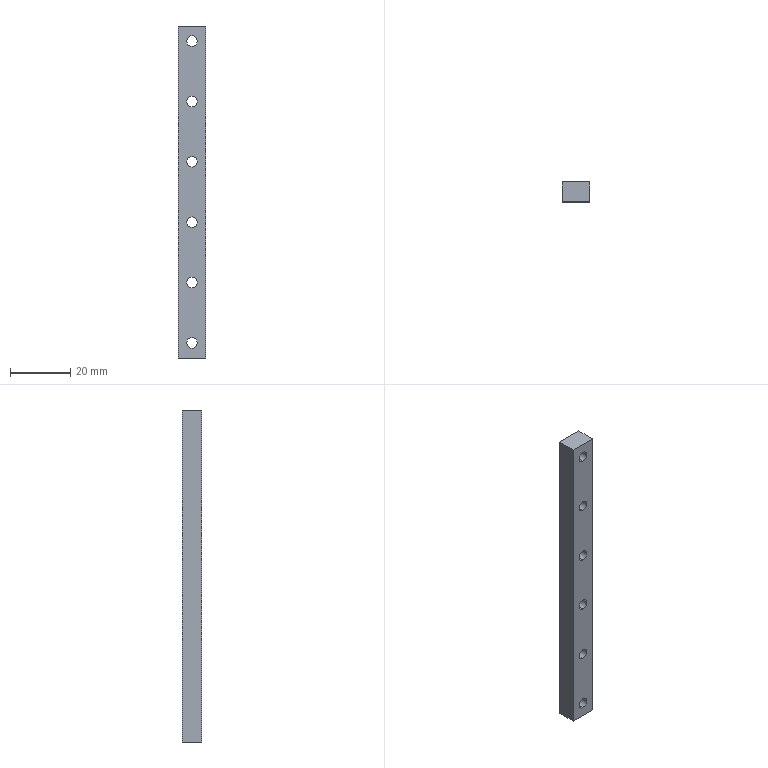Part | STEP file | Mount electronic clip sMGN9C110 | 1 solid | 36 faces | box 9 x 6.5 x 110 mm | volume 5668 mm3 | cylinder 24 | plane 12 | commonest cylinder face diameters 3.5 x12 6 x12